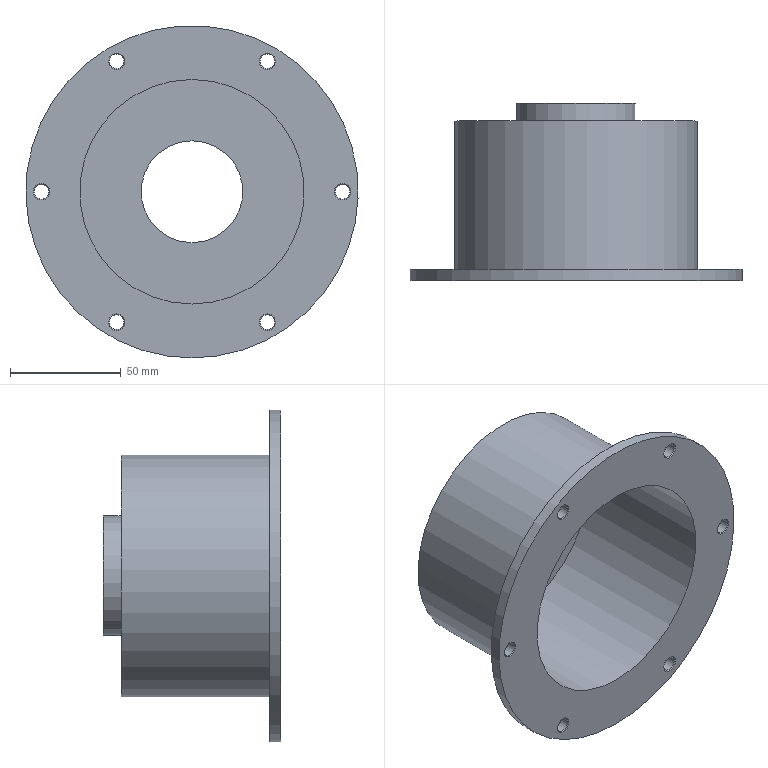Part | NX | features DATUM_CSYS 8, SKETCH 7, EXTRACT_DATUM_AXIS 6, EXTRACT_FACE 6, HOLE PACKAGE 6, SIMPLE HOLE 6, Instance Feature 5, Pattern Feature 1, SWP104 1 | 1 solid | 28 faces | box 150 x 80 x 150 mm | volume 166346 mm3 | cone 12 | cylinder 11 | plane 5 | commonest cylinder face diameters 6.6 x6 46 x1 54 x1 101.387 x1 109.387 x1 150 x1
STEP:
#1=CARTESIAN_POINT('',(0.,72.,-54.693));
#2=VERTEX_POINT('',#1);
#3=CARTESIAN_POINT('',(0.,72.,0.));
#4=DIRECTION('',(0.,-1.,0.));
#5=DIRECTION('',(0.,0.,-1.));
#6=AXIS2_PLACEMENT_3D('',#3,#4,#5);
#7=CIRCLE('',#6,54.693);
#8=EDGE_CURVE('',#2,#2,#7,.T.);
#9=ORIENTED_EDGE('',*,*,#8,.T.);
#10=EDGE_LOOP('',(#9));
#11=FACE_BOUND('',#10,.T.);
#12=CARTESIAN_POINT('',(0.,5.,-54.693));
#13=VERTEX_POINT('',#12);
#14=CARTESIAN_POINT('',(0.,5.,0.));
#15=DIRECTION('',(0.,-1.,0.));
#16=DIRECTION('',(0.,0.,-1.));
#17=AXIS2_PLACEMENT_3D('',#14,#15,#16);
#18=CIRCLE('',#17,54.693);
#19=EDGE_CURVE('',#13,#13,#18,.T.);
#20=ORIENTED_EDGE('',*,*,#19,.F.);
#21=EDGE_LOOP('',(#20));
#22=FACE_BOUND('',#21,.T.);
#23=CARTESIAN_POINT('',(0.,0.,0.));
#24=DIRECTION('',(0.,-1.,0.));
#25=DIRECTION('',(0.,0.,-1.));
#26=AXIS2_PLACEMENT_3D('',#23,#24,#25);
#27=CYLINDRICAL_SURFACE('',#26,54.693);
#28=ADVANCED_FACE('',(#11,#22),#27,.T.);
#29=CARTESIAN_POINT('',(0.,72.,-27.));
#30=VERTEX_POINT('',#29);
#31=CARTESIAN_POINT('',(0.,72.,0.));
#32=DIRECTION('',(0.,-1.,0.));
#33=DIRECTION('',(0.,0.,-1.));
#34=AXIS2_PLACEMENT_3D('',#31,#32,#33);
#35=CIRCLE('',#34,27.);
#36=EDGE_CURVE('',#30,#30,#35,.T.);
#37=ORIENTED_EDGE('',*,*,#36,.T.);
#38=EDGE_LOOP('',(#37));
#39=FACE_BOUND('',#38,.T.);
#40=ORIENTED_EDGE('',*,*,#8,.F.);
#41=EDGE_LOOP('',(#40));
#42=FACE_BOUND('',#41,.T.);
#43=CARTESIAN_POINT('',(54.693,72.,0.));
#44=DIRECTION('',(0.,1.,0.));
#45=DIRECTION('',(0.,0.,1.));
#46=AXIS2_PLACEMENT_3D('',#43,#44,#45);
#47=PLANE('',#46);
#48=ADVANCED_FACE('',(#39,#42),#47,.T.);
#49=CARTESIAN_POINT('',(0.,80.,-27.));
#50=VERTEX_POINT('',#49);
#51=CARTESIAN_POINT('',(0.,80.,0.));
#52=DIRECTION('',(0.,-1.,0.));
#53=DIRECTION('',(0.,0.,-1.));
#54=AXIS2_PLACEMENT_3D('',#51,#52,#53);
#55=CIRCLE('',#54,27.);
#56=EDGE_CURVE('',#50,#50,#55,.T.);
#57=ORIENTED_EDGE('',*,*,#56,.T.);
#58=EDGE_LOOP('',(#57));
#59=FACE_BOUND('',#58,.T.);
#60=ORIENTED_EDGE('',*,*,#36,.F.);
#61=EDGE_LOOP('',(#60));
#62=FACE_BOUND('',#61,.T.);
#63=CARTESIAN_POINT('',(0.,0.,0.));
#64=DIRECTION('',(0.,-1.,0.));
#65=DIRECTION('',(0.,0.,-1.));
#66=AXIS2_PLACEMENT_3D('',#63,#64,#65);
#67=CYLINDRICAL_SURFACE('',#66,27.);
#68=ADVANCED_FACE('',(#59,#62),#67,.T.);
#69=CARTESIAN_POINT('',(0.,80.,-23.));
#70=VERTEX_POINT('',#69);
#71=CARTESIAN_POINT('',(0.,80.,0.));
#72=DIRECTION('',(0.,-1.,0.));
#73=DIRECTION('',(0.,0.,-1.));
#74=AXIS2_PLACEMENT_3D('',#71,#72,#73);
#75=CIRCLE('',#74,23.);
#76=EDGE_CURVE('',#70,#70,#75,.T.);
#77=ORIENTED_EDGE('',*,*,#76,.T.);
#78=EDGE_LOOP('',(#77));
#79=FACE_BOUND('',#78,.T.);
#80=ORIENTED_EDGE('',*,*,#56,.F.);
#81=EDGE_LOOP('',(#80));
#82=FACE_BOUND('',#81,.T.);
#83=CARTESIAN_POINT('',(27.,80.,0.));
#84=DIRECTION('',(0.,1.,0.));
#85=DIRECTION('',(0.,0.,1.));
#86=AXIS2_PLACEMENT_3D('',#83,#84,#85);
#87=PLANE('',#86);
#88=ADVANCED_FACE('',(#79,#82),#87,.T.);
#89=CARTESIAN_POINT('',(0.,68.,-23.));
#90=VERTEX_POINT('',#89);
#91=CARTESIAN_POINT('',(0.,68.,0.));
#92=DIRECTION('',(0.,-1.,0.));
#93=DIRECTION('',(0.,0.,-1.));
#94=AXIS2_PLACEMENT_3D('',#91,#92,#93);
#95=CIRCLE('',#94,23.);
#96=EDGE_CURVE('',#90,#90,#95,.T.);
#97=ORIENTED_EDGE('',*,*,#96,.T.);
#98=EDGE_LOOP('',(#97));
#99=FACE_BOUND('',#98,.T.);
#100=ORIENTED_EDGE('',*,*,#76,.F.);
#101=EDGE_LOOP('',(#100));
#102=FACE_BOUND('',#101,.T.);
#103=CARTESIAN_POINT('',(0.,0.,0.));
#104=DIRECTION('',(0.,-1.,0.));
#105=DIRECTION('',(0.,0.,-1.));
#106=AXIS2_PLACEMENT_3D('',#103,#104,#105);
#107=CYLINDRICAL_SURFACE('',#106,23.);
#108=ADVANCED_FACE('',(#99,#102),#107,.F.);
#109=CARTESIAN_POINT('',(0.,68.,-50.693));
#110=VERTEX_POINT('',#109);
#111=CARTESIAN_POINT('',(0.,68.,0.));
#112=DIRECTION('',(0.,-1.,0.));
#113=DIRECTION('',(0.,0.,-1.));
#114=AXIS2_PLACEMENT_3D('',#111,#112,#113);
#115=CIRCLE('',#114,50.693);
#116=EDGE_CURVE('',#110,#110,#115,.T.);
#117=ORIENTED_EDGE('',*,*,#116,.T.);
#118=EDGE_LOOP('',(#117));
#119=FACE_BOUND('',#118,.T.);
#120=ORIENTED_EDGE('',*,*,#96,.F.);
#121=EDGE_LOOP('',(#120));
#122=FACE_BOUND('',#121,.T.);
#123=CARTESIAN_POINT('',(23.,68.,0.));
#124=DIRECTION('',(0.,-1.,0.));
#125=DIRECTION('',(0.,0.,-1.));
#126=AXIS2_PLACEMENT_3D('',#123,#124,#125);
#127=PLANE('',#126);
#128=ADVANCED_FACE('',(#119,#122),#127,.T.);
#129=CARTESIAN_POINT('',(0.,0.,-50.693));
#130=VERTEX_POINT('',#129);
#131=CARTESIAN_POINT('',(0.,0.,0.));
#132=DIRECTION('',(0.,-1.,0.));
#133=DIRECTION('',(0.,0.,-1.));
#134=AXIS2_PLACEMENT_3D('',#131,#132,#133);
#135=CIRCLE('',#134,50.693);
#136=EDGE_CURVE('',#130,#130,#135,.T.);
#137=ORIENTED_EDGE('',*,*,#136,.T.);
#138=EDGE_LOOP('',(#137));
#139=FACE_BOUND('',#138,.T.);
#140=ORIENTED_EDGE('',*,*,#116,.F.);
#141=EDGE_LOOP('',(#140));
#142=FACE_BOUND('',#141,.T.);
#143=CARTESIAN_POINT('',(0.,0.,0.));
#144=DIRECTION('',(0.,-1.,0.));
#145=DIRECTION('',(0.,0.,-1.));
#146=AXIS2_PLACEMENT_3D('',#143,#144,#145);
#147=CYLINDRICAL_SURFACE('',#146,50.693);
#148=ADVANCED_FACE('',(#139,#142),#147,.F.);
#149=CARTESIAN_POINT('',(34.,0.,55.19));
#150=VERTEX_POINT('',#149);
#151=CARTESIAN_POINT('',(34.,0.,58.89));
#152=DIRECTION('',(0.,-1.,0.));
#153=DIRECTION('',(0.,0.,-1.));
#154=AXIS2_PLACEMENT_3D('',#151,#152,#153);
#155=CIRCLE('',#154,3.7);
#156=EDGE_CURVE('',#150,#150,#155,.F.);
#157=ORIENTED_EDGE('',*,*,#156,.T.);
#158=EDGE_LOOP('',(#157));
#159=FACE_BOUND('',#158,.T.);
#160=CARTESIAN_POINT('',(-34.,0.,55.19));
#161=VERTEX_POINT('',#160);
#162=CARTESIAN_POINT('',(-34.,0.,58.89));
#163=DIRECTION('',(0.,-1.,0.));
#164=DIRECTION('',(0.,0.,-1.));
#165=AXIS2_PLACEMENT_3D('',#162,#163,#164);
#166=CIRCLE('',#165,3.7);
#167=EDGE_CURVE('',#161,#161,#166,.F.);
#168=ORIENTED_EDGE('',*,*,#167,.T.);
#169=EDGE_LOOP('',(#168));
#170=FACE_BOUND('',#169,.T.);
#171=CARTESIAN_POINT('',(-68.,0.,-3.7));
#172=VERTEX_POINT('',#171);
#173=CARTESIAN_POINT('',(-68.,0.,0.));
#174=DIRECTION('',(0.,-1.,0.));
#175=DIRECTION('',(0.,0.,-1.));
#176=AXIS2_PLACEMENT_3D('',#173,#174,#175);
#177=CIRCLE('',#176,3.7);
#178=EDGE_CURVE('',#172,#172,#177,.F.);
#179=ORIENTED_EDGE('',*,*,#178,.T.);
#180=EDGE_LOOP('',(#179));
#181=FACE_BOUND('',#180,.T.);
#182=CARTESIAN_POINT('',(-34.,0.,-62.59));
#183=VERTEX_POINT('',#182);
#184=CARTESIAN_POINT('',(-34.,0.,-58.89));
#185=DIRECTION('',(0.,-1.,0.));
#186=DIRECTION('',(0.,0.,-1.));
#187=AXIS2_PLACEMENT_3D('',#184,#185,#186);
#188=CIRCLE('',#187,3.7);
#189=EDGE_CURVE('',#183,#183,#188,.F.);
#190=ORIENTED_EDGE('',*,*,#189,.T.);
#191=EDGE_LOOP('',(#190));
#192=FACE_BOUND('',#191,.T.);
#193=CARTESIAN_POINT('',(34.,0.,-62.59));
#194=VERTEX_POINT('',#193);
#195=CARTESIAN_POINT('',(34.,0.,-58.89));
#196=DIRECTION('',(0.,-1.,0.));
#197=DIRECTION('',(0.,0.,-1.));
#198=AXIS2_PLACEMENT_3D('',#195,#196,#197);
#199=CIRCLE('',#198,3.7);
#200=EDGE_CURVE('',#194,#194,#199,.F.);
#201=ORIENTED_EDGE('',*,*,#200,.T.);
#202=EDGE_LOOP('',(#201));
#203=FACE_BOUND('',#202,.T.);
#204=CARTESIAN_POINT('',(68.,0.,-3.7));
#205=VERTEX_POINT('',#204);
#206=CARTESIAN_POINT('',(68.,0.,0.));
#207=DIRECTION('',(0.,-1.,0.));
#208=DIRECTION('',(0.,0.,-1.));
#209=AXIS2_PLACEMENT_3D('',#206,#207,#208);
#210=CIRCLE('',#209,3.7);
#211=EDGE_CURVE('',#205,#205,#210,.F.);
#212=ORIENTED_EDGE('',*,*,#211,.T.);
#213=EDGE_LOOP('',(#212));
#214=FACE_BOUND('',#213,.T.);
#215=CARTESIAN_POINT('',(0.,0.,-75.));
#216=VERTEX_POINT('',#215);
#217=CARTESIAN_POINT('',(0.,0.,0.));
#218=DIRECTION('',(0.,-1.,0.));
#219=DIRECTION('',(0.,0.,-1.));
#220=AXIS2_PLACEMENT_3D('',#217,#218,#219);
#221=CIRCLE('',#220,75.);
#222=EDGE_CURVE('',#216,#216,#221,.T.);
#223=ORIENTED_EDGE('',*,*,#222,.T.);
#224=EDGE_LOOP('',(#223));
#225=FACE_BOUND('',#224,.T.);
#226=ORIENTED_EDGE('',*,*,#136,.F.);
#227=EDGE_LOOP('',(#226));
#228=FACE_BOUND('',#227,.T.);
#229=CARTESIAN_POINT('',(50.693,0.,0.));
#230=DIRECTION('',(0.,-1.,0.));
#231=DIRECTION('',(0.,0.,-1.));
#232=AXIS2_PLACEMENT_3D('',#229,#230,#231);
#233=PLANE('',#232);
#234=ADVANCED_FACE('',(#159,#170,#181,#192,#203,#214,#225,#228),#233,.T.);
#235=CARTESIAN_POINT('',(0.,5.,-75.));
#236=VERTEX_POINT('',#235);
#237=CARTESIAN_POINT('',(0.,5.,0.));
#238=DIRECTION('',(0.,-1.,0.));
#239=DIRECTION('',(0.,0.,-1.));
#240=AXIS2_PLACEMENT_3D('',#237,#238,#239);
#241=CIRCLE('',#240,75.);
#242=EDGE_CURVE('',#236,#236,#241,.T.);
#243=ORIENTED_EDGE('',*,*,#242,.T.);
#244=EDGE_LOOP('',(#243));
#245=FACE_BOUND('',#244,.T.);
#246=ORIENTED_EDGE('',*,*,#222,.F.);
#247=EDGE_LOOP('',(#246));
#248=FACE_BOUND('',#247,.T.);
#249=CARTESIAN_POINT('',(0.,0.,0.));
#250=DIRECTION('',(0.,-1.,0.));
#251=DIRECTION('',(0.,0.,-1.));
#252=AXIS2_PLACEMENT_3D('',#249,#250,#251);
#253=CYLINDRICAL_SURFACE('',#252,75.);
#254=ADVANCED_FACE('',(#245,#248),#253,.T.);
#255=CARTESIAN_POINT('',(34.,5.,62.59));
#256=VERTEX_POINT('',#255);
#257=CARTESIAN_POINT('',(34.,5.,58.89));
#258=DIRECTION('',(0.,1.,0.));
#259=DIRECTION('',(0.,0.,1.));
#260=AXIS2_PLACEMENT_3D('',#257,#258,#259);
#261=CIRCLE('',#260,3.7);
#262=EDGE_CURVE('',#256,#256,#261,.F.);
#263=ORIENTED_EDGE('',*,*,#262,.T.);
#264=EDGE_LOOP('',(#263));
#265=FACE_BOUND('',#264,.T.);
#266=CARTESIAN_POINT('',(-34.,5.,62.59));
#267=VERTEX_POINT('',#266);
#268=CARTESIAN_POINT('',(-34.,5.,58.89));
#269=DIRECTION('',(0.,1.,0.));
#270=DIRECTION('',(0.,0.,1.));
#271=AXIS2_PLACEMENT_3D('',#268,#269,#270);
#272=CIRCLE('',#271,3.7);
#273=EDGE_CURVE('',#267,#267,#272,.F.);
#274=ORIENTED_EDGE('',*,*,#273,.T.);
#275=EDGE_LOOP('',(#274));
#276=FACE_BOUND('',#275,.T.);
#277=CARTESIAN_POINT('',(-68.,5.,3.7));
#278=VERTEX_POINT('',#277);
#279=CARTESIAN_POINT('',(-68.,5.,0.));
#280=DIRECTION('',(0.,1.,0.));
#281=DIRECTION('',(0.,0.,1.));
#282=AXIS2_PLACEMENT_3D('',#279,#280,#281);
#283=CIRCLE('',#282,3.7);
#284=EDGE_CURVE('',#278,#278,#283,.F.);
#285=ORIENTED_EDGE('',*,*,#284,.T.);
#286=EDGE_LOOP('',(#285));
#287=FACE_BOUND('',#286,.T.);
#288=CARTESIAN_POINT('',(-34.,5.,-55.19));
#289=VERTEX_POINT('',#288);
#290=CARTESIAN_POINT('',(-34.,5.,-58.89));
#291=DIRECTION('',(0.,1.,0.));
#292=DIRECTION('',(0.,0.,1.));
#293=AXIS2_PLACEMENT_3D('',#290,#291,#292);
#294=CIRCLE('',#293,3.7);
#295=EDGE_CURVE('',#289,#289,#294,.F.);
#296=ORIENTED_EDGE('',*,*,#295,.T.);
#297=EDGE_LOOP('',(#296));
#298=FACE_BOUND('',#297,.T.);
#299=CARTESIAN_POINT('',(34.,5.,-55.19));
#300=VERTEX_POINT('',#299);
#301=CARTESIAN_POINT('',(34.,5.,-58.89));
#302=DIRECTION('',(0.,1.,0.));
#303=DIRECTION('',(0.,0.,1.));
#304=AXIS2_PLACEMENT_3D('',#301,#302,#303);
#305=CIRCLE('',#304,3.7);
#306=EDGE_CURVE('',#300,#300,#305,.F.);
#307=ORIENTED_EDGE('',*,*,#306,.T.);
#308=EDGE_LOOP('',(#307));
#309=FACE_BOUND('',#308,.T.);
#310=CARTESIAN_POINT('',(68.,5.,3.7));
#311=VERTEX_POINT('',#310);
#312=CARTESIAN_POINT('',(68.,5.,0.));
#313=DIRECTION('',(0.,1.,0.));
#314=DIRECTION('',(0.,0.,1.));
#315=AXIS2_PLACEMENT_3D('',#312,#313,#314);
#316=CIRCLE('',#315,3.7);
#317=EDGE_CURVE('',#311,#311,#316,.F.);
#318=ORIENTED_EDGE('',*,*,#317,.T.);
#319=EDGE_LOOP('',(#318));
#320=FACE_BOUND('',#319,.T.);
#321=ORIENTED_EDGE('',*,*,#19,.T.);
#322=EDGE_LOOP('',(#321));
#323=FACE_BOUND('',#322,.T.);
#324=ORIENTED_EDGE('',*,*,#242,.F.);
#325=EDGE_LOOP('',(#324));
#326=FACE_BOUND('',#325,.T.);
#327=CARTESIAN_POINT('',(75.,5.,0.));
#328=DIRECTION('',(0.,1.,0.));
#329=DIRECTION('',(0.,0.,1.));
#330=AXIS2_PLACEMENT_3D('',#327,#328,#329);
#331=PLANE('',#330);
#332=ADVANCED_FACE('',(#265,#276,#287,#298,#309,#320,#323,#326),#331,.T.);
#333=CARTESIAN_POINT('',(68.,0.4,-3.3));
#334=VERTEX_POINT('',#333);
#335=CARTESIAN_POINT('',(68.,0.4,0.));
#336=DIRECTION('',(0.,-1.,0.));
#337=DIRECTION('',(0.,0.,-1.));
#338=AXIS2_PLACEMENT_3D('',#335,#336,#337);
#339=CIRCLE('',#338,3.3);
#340=EDGE_CURVE('',#334,#334,#339,.T.);
#341=ORIENTED_EDGE('',*,*,#340,.T.);
#342=EDGE_LOOP('',(#341));
#343=FACE_BOUND('',#342,.T.);
#344=CARTESIAN_POINT('',(68.,4.6,3.3));
#345=VERTEX_POINT('',#344);
#346=CARTESIAN_POINT('',(68.,4.6,0.));
#347=DIRECTION('',(0.,1.,0.));
#348=DIRECTION('',(0.,0.,1.));
#349=AXIS2_PLACEMENT_3D('',#346,#347,#348);
#350=CIRCLE('',#349,3.3);
#351=EDGE_CURVE('',#345,#345,#350,.T.);
#352=ORIENTED_EDGE('',*,*,#351,.T.);
#353=EDGE_LOOP('',(#352));
#354=FACE_BOUND('',#353,.T.);
#355=CARTESIAN_POINT('',(68.,5.,0.));
#356=DIRECTION('',(0.,-1.,0.));
#357=DIRECTION('',(0.,0.,-1.));
#358=AXIS2_PLACEMENT_3D('',#355,#356,#357);
#359=CYLINDRICAL_SURFACE('',#358,3.3);
#360=ADVANCED_FACE('',(#343,#354),#359,.F.);
#361=ORIENTED_EDGE('',*,*,#351,.F.);
#362=EDGE_LOOP('',(#361));
#363=FACE_BOUND('',#362,.T.);
#364=ORIENTED_EDGE('',*,*,#317,.F.);
#365=EDGE_LOOP('',(#364));
#366=FACE_BOUND('',#365,.T.);
#367=CARTESIAN_POINT('',(68.,5.,0.));
#368=DIRECTION('',(0.,1.,0.));
#369=DIRECTION('',(0.,0.,1.));
#370=AXIS2_PLACEMENT_3D('',#367,#368,#369);
#371=CONICAL_SURFACE('',#370,3.7,0.7854);
#372=ADVANCED_FACE('',(#363,#366),#371,.F.);
#373=ORIENTED_EDGE('',*,*,#211,.F.);
#374=EDGE_LOOP('',(#373));
#375=FACE_BOUND('',#374,.T.);
#376=ORIENTED_EDGE('',*,*,#340,.F.);
#377=EDGE_LOOP('',(#376));
#378=FACE_BOUND('',#377,.T.);
#379=CARTESIAN_POINT('',(68.,0.4,0.));
#380=DIRECTION('',(0.,-1.,0.));
#381=DIRECTION('',(0.,0.,-1.));
#382=AXIS2_PLACEMENT_3D('',#379,#380,#381);
#383=CONICAL_SURFACE('',#382,3.3,0.7854);
#384=ADVANCED_FACE('',(#375,#378),#383,.F.);
#385=CARTESIAN_POINT('',(34.,0.4,-62.19));
#386=VERTEX_POINT('',#385);
#387=CARTESIAN_POINT('',(34.,0.4,-58.89));
#388=DIRECTION('',(0.,-1.,0.));
#389=DIRECTION('',(0.,0.,-1.));
#390=AXIS2_PLACEMENT_3D('',#387,#388,#389);
#391=CIRCLE('',#390,3.3);
#392=EDGE_CURVE('',#386,#386,#391,.T.);
#393=ORIENTED_EDGE('',*,*,#392,.T.);
#394=EDGE_LOOP('',(#393));
#395=FACE_BOUND('',#394,.T.);
#396=CARTESIAN_POINT('',(34.,4.6,-55.59));
#397=VERTEX_POINT('',#396);
#398=CARTESIAN_POINT('',(34.,4.6,-58.89));
#399=DIRECTION('',(0.,1.,0.));
#400=DIRECTION('',(0.,0.,1.));
#401=AXIS2_PLACEMENT_3D('',#398,#399,#400);
#402=CIRCLE('',#401,3.3);
#403=EDGE_CURVE('',#397,#397,#402,.T.);
#404=ORIENTED_EDGE('',*,*,#403,.T.);
#405=EDGE_LOOP('',(#404));
#406=FACE_BOUND('',#405,.T.);
#407=CARTESIAN_POINT('',(34.,5.,-58.89));
#408=DIRECTION('',(0.,-1.,0.));
#409=DIRECTION('',(0.,0.,-1.));
#410=AXIS2_PLACEMENT_3D('',#407,#408,#409);
#411=CYLINDRICAL_SURFACE('',#410,3.3);
#412=ADVANCED_FACE('',(#395,#406),#411,.F.);
#413=ORIENTED_EDGE('',*,*,#403,.F.);
#414=EDGE_LOOP('',(#413));
#415=FACE_BOUND('',#414,.T.);
#416=ORIENTED_EDGE('',*,*,#306,.F.);
#417=EDGE_LOOP('',(#416));
#418=FACE_BOUND('',#417,.T.);
#419=CARTESIAN_POINT('',(34.,5.,-58.89));
#420=DIRECTION('',(0.,1.,0.));
#421=DIRECTION('',(0.,0.,1.));
#422=AXIS2_PLACEMENT_3D('',#419,#420,#421);
#423=CONICAL_SURFACE('',#422,3.7,0.7854);
#424=ADVANCED_FACE('',(#415,#418),#423,.F.);
#425=ORIENTED_EDGE('',*,*,#200,.F.);
#426=EDGE_LOOP('',(#425));
#427=FACE_BOUND('',#426,.T.);
#428=ORIENTED_EDGE('',*,*,#392,.F.);
#429=EDGE_LOOP('',(#428));
#430=FACE_BOUND('',#429,.T.);
#431=CARTESIAN_POINT('',(34.,0.4,-58.89));
#432=DIRECTION('',(0.,-1.,0.));
#433=DIRECTION('',(0.,0.,-1.));
#434=AXIS2_PLACEMENT_3D('',#431,#432,#433);
#435=CONICAL_SURFACE('',#434,3.3,0.7854);
#436=ADVANCED_FACE('',(#427,#430),#435,.F.);
#437=CARTESIAN_POINT('',(-34.,0.4,-62.19));
#438=VERTEX_POINT('',#437);
#439=CARTESIAN_POINT('',(-34.,0.4,-58.89));
#440=DIRECTION('',(0.,-1.,0.));
#441=DIRECTION('',(0.,0.,-1.));
#442=AXIS2_PLACEMENT_3D('',#439,#440,#441);
#443=CIRCLE('',#442,3.3);
#444=EDGE_CURVE('',#438,#438,#443,.T.);
#445=ORIENTED_EDGE('',*,*,#444,.T.);
#446=EDGE_LOOP('',(#445));
#447=FACE_BOUND('',#446,.T.);
#448=CARTESIAN_POINT('',(-34.,4.6,-55.59));
#449=VERTEX_POINT('',#448);
#450=CARTESIAN_POINT('',(-34.,4.6,-58.89));
#451=DIRECTION('',(0.,1.,0.));
#452=DIRECTION('',(0.,0.,1.));
#453=AXIS2_PLACEMENT_3D('',#450,#451,#452);
#454=CIRCLE('',#453,3.3);
#455=EDGE_CURVE('',#449,#449,#454,.T.);
#456=ORIENTED_EDGE('',*,*,#455,.T.);
#457=EDGE_LOOP('',(#456));
#458=FACE_BOUND('',#457,.T.);
#459=CARTESIAN_POINT('',(-34.,5.,-58.89));
#460=DIRECTION('',(0.,-1.,0.));
#461=DIRECTION('',(0.,0.,-1.));
#462=AXIS2_PLACEMENT_3D('',#459,#460,#461);
#463=CYLINDRICAL_SURFACE('',#462,3.3);
#464=ADVANCED_FACE('',(#447,#458),#463,.F.);
#465=ORIENTED_EDGE('',*,*,#455,.F.);
#466=EDGE_LOOP('',(#465));
#467=FACE_BOUND('',#466,.T.);
#468=ORIENTED_EDGE('',*,*,#295,.F.);
#469=EDGE_LOOP('',(#468));
#470=FACE_BOUND('',#469,.T.);
#471=CARTESIAN_POINT('',(-34.,5.,-58.89));
#472=DIRECTION('',(0.,1.,0.));
#473=DIRECTION('',(0.,0.,1.));
#474=AXIS2_PLACEMENT_3D('',#471,#472,#473);
#475=CONICAL_SURFACE('',#474,3.7,0.7854);
#476=ADVANCED_FACE('',(#467,#470),#475,.F.);
#477=ORIENTED_EDGE('',*,*,#189,.F.);
#478=EDGE_LOOP('',(#477));
#479=FACE_BOUND('',#478,.T.);
#480=ORIENTED_EDGE('',*,*,#444,.F.);
#481=EDGE_LOOP('',(#480));
#482=FACE_BOUND('',#481,.T.);
#483=CARTESIAN_POINT('',(-34.,0.4,-58.89));
#484=DIRECTION('',(0.,-1.,0.));
#485=DIRECTION('',(0.,0.,-1.));
#486=AXIS2_PLACEMENT_3D('',#483,#484,#485);
#487=CONICAL_SURFACE('',#486,3.3,0.7854);
#488=ADVANCED_FACE('',(#479,#482),#487,.F.);
#489=CARTESIAN_POINT('',(-68.,0.4,-3.3));
#490=VERTEX_POINT('',#489);
#491=CARTESIAN_POINT('',(-68.,0.4,0.));
#492=DIRECTION('',(0.,-1.,0.));
#493=DIRECTION('',(0.,0.,-1.));
#494=AXIS2_PLACEMENT_3D('',#491,#492,#493);
#495=CIRCLE('',#494,3.3);
#496=EDGE_CURVE('',#490,#490,#495,.T.);
#497=ORIENTED_EDGE('',*,*,#496,.T.);
#498=EDGE_LOOP('',(#497));
#499=FACE_BOUND('',#498,.T.);
#500=CARTESIAN_POINT('',(-68.,4.6,3.3));
#501=VERTEX_POINT('',#500);
#502=CARTESIAN_POINT('',(-68.,4.6,0.));
#503=DIRECTION('',(0.,1.,0.));
#504=DIRECTION('',(0.,0.,1.));
#505=AXIS2_PLACEMENT_3D('',#502,#503,#504);
#506=CIRCLE('',#505,3.3);
#507=EDGE_CURVE('',#501,#501,#506,.T.);
#508=ORIENTED_EDGE('',*,*,#507,.T.);
#509=EDGE_LOOP('',(#508));
#510=FACE_BOUND('',#509,.T.);
#511=CARTESIAN_POINT('',(-68.,5.,0.));
#512=DIRECTION('',(0.,-1.,0.));
#513=DIRECTION('',(0.,0.,-1.));
#514=AXIS2_PLACEMENT_3D('',#511,#512,#513);
#515=CYLINDRICAL_SURFACE('',#514,3.3);
#516=ADVANCED_FACE('',(#499,#510),#515,.F.);
#517=ORIENTED_EDGE('',*,*,#507,.F.);
#518=EDGE_LOOP('',(#517));
#519=FACE_BOUND('',#518,.T.);
#520=ORIENTED_EDGE('',*,*,#284,.F.);
#521=EDGE_LOOP('',(#520));
#522=FACE_BOUND('',#521,.T.);
#523=CARTESIAN_POINT('',(-68.,5.,0.));
#524=DIRECTION('',(0.,1.,0.));
#525=DIRECTION('',(0.,0.,1.));
#526=AXIS2_PLACEMENT_3D('',#523,#524,#525);
#527=CONICAL_SURFACE('',#526,3.7,0.7854);
#528=ADVANCED_FACE('',(#519,#522),#527,.F.);
#529=ORIENTED_EDGE('',*,*,#178,.F.);
#530=EDGE_LOOP('',(#529));
#531=FACE_BOUND('',#530,.T.);
#532=ORIENTED_EDGE('',*,*,#496,.F.);
#533=EDGE_LOOP('',(#532));
#534=FACE_BOUND('',#533,.T.);
#535=CARTESIAN_POINT('',(-68.,0.4,0.));
#536=DIRECTION('',(0.,-1.,0.));
#537=DIRECTION('',(0.,0.,-1.));
#538=AXIS2_PLACEMENT_3D('',#535,#536,#537);
#539=CONICAL_SURFACE('',#538,3.3,0.7854);
#540=ADVANCED_FACE('',(#531,#534),#539,.F.);
#541=CARTESIAN_POINT('',(-34.,0.4,55.59));
#542=VERTEX_POINT('',#541);
#543=CARTESIAN_POINT('',(-34.,0.4,58.89));
#544=DIRECTION('',(0.,-1.,0.));
#545=DIRECTION('',(0.,0.,-1.));
#546=AXIS2_PLACEMENT_3D('',#543,#544,#545);
#547=CIRCLE('',#546,3.3);
#548=EDGE_CURVE('',#542,#542,#547,.T.);
#549=ORIENTED_EDGE('',*,*,#548,.T.);
#550=EDGE_LOOP('',(#549));
#551=FACE_BOUND('',#550,.T.);
#552=CARTESIAN_POINT('',(-34.,4.6,62.19));
#553=VERTEX_POINT('',#552);
#554=CARTESIAN_POINT('',(-34.,4.6,58.89));
#555=DIRECTION('',(0.,1.,0.));
#556=DIRECTION('',(0.,0.,1.));
#557=AXIS2_PLACEMENT_3D('',#554,#555,#556);
#558=CIRCLE('',#557,3.3);
#559=EDGE_CURVE('',#553,#553,#558,.T.);
#560=ORIENTED_EDGE('',*,*,#559,.T.);
#561=EDGE_LOOP('',(#560));
#562=FACE_BOUND('',#561,.T.);
#563=CARTESIAN_POINT('',(-34.,5.,58.89));
#564=DIRECTION('',(0.,-1.,0.));
#565=DIRECTION('',(0.,0.,-1.));
#566=AXIS2_PLACEMENT_3D('',#563,#564,#565);
#567=CYLINDRICAL_SURFACE('',#566,3.3);
#568=ADVANCED_FACE('',(#551,#562),#567,.F.);
#569=ORIENTED_EDGE('',*,*,#559,.F.);
#570=EDGE_LOOP('',(#569));
#571=FACE_BOUND('',#570,.T.);
#572=ORIENTED_EDGE('',*,*,#273,.F.);
#573=EDGE_LOOP('',(#572));
#574=FACE_BOUND('',#573,.T.);
#575=CARTESIAN_POINT('',(-34.,5.,58.89));
#576=DIRECTION('',(0.,1.,0.));
#577=DIRECTION('',(0.,0.,1.));
#578=AXIS2_PLACEMENT_3D('',#575,#576,#577);
#579=CONICAL_SURFACE('',#578,3.7,0.7854);
#580=ADVANCED_FACE('',(#571,#574),#579,.F.);
#581=ORIENTED_EDGE('',*,*,#167,.F.);
#582=EDGE_LOOP('',(#581));
#583=FACE_BOUND('',#582,.T.);
#584=ORIENTED_EDGE('',*,*,#548,.F.);
#585=EDGE_LOOP('',(#584));
#586=FACE_BOUND('',#585,.T.);
#587=CARTESIAN_POINT('',(-34.,0.4,58.89));
#588=DIRECTION('',(0.,-1.,0.));
#589=DIRECTION('',(0.,0.,-1.));
#590=AXIS2_PLACEMENT_3D('',#587,#588,#589);
#591=CONICAL_SURFACE('',#590,3.3,0.7854);
#592=ADVANCED_FACE('',(#583,#586),#591,.F.);
#593=CARTESIAN_POINT('',(34.,0.4,55.59));
#594=VERTEX_POINT('',#593);
#595=CARTESIAN_POINT('',(34.,0.4,58.89));
#596=DIRECTION('',(0.,-1.,0.));
#597=DIRECTION('',(0.,0.,-1.));
#598=AXIS2_PLACEMENT_3D('',#595,#596,#597);
#599=CIRCLE('',#598,3.3);
#600=EDGE_CURVE('',#594,#594,#599,.T.);
#601=ORIENTED_EDGE('',*,*,#600,.T.);
#602=EDGE_LOOP('',(#601));
#603=FACE_BOUND('',#602,.T.);
#604=CARTESIAN_POINT('',(34.,4.6,62.19));
#605=VERTEX_POINT('',#604);
#606=CARTESIAN_POINT('',(34.,4.6,58.89));
#607=DIRECTION('',(0.,1.,0.));
#608=DIRECTION('',(0.,0.,1.));
#609=AXIS2_PLACEMENT_3D('',#606,#607,#608);
#610=CIRCLE('',#609,3.3);
#611=EDGE_CURVE('',#605,#605,#610,.T.);
#612=ORIENTED_EDGE('',*,*,#611,.T.);
#613=EDGE_LOOP('',(#612));
#614=FACE_BOUND('',#613,.T.);
#615=CARTESIAN_POINT('',(34.,5.,58.89));
#616=DIRECTION('',(0.,-1.,0.));
#617=DIRECTION('',(0.,0.,-1.));
#618=AXIS2_PLACEMENT_3D('',#615,#616,#617);
#619=CYLINDRICAL_SURFACE('',#618,3.3);
#620=ADVANCED_FACE('',(#603,#614),#619,.F.);
#621=ORIENTED_EDGE('',*,*,#611,.F.);
#622=EDGE_LOOP('',(#621));
#623=FACE_BOUND('',#622,.T.);
#624=ORIENTED_EDGE('',*,*,#262,.F.);
#625=EDGE_LOOP('',(#624));
#626=FACE_BOUND('',#625,.T.);
#627=CARTESIAN_POINT('',(34.,5.,58.89));
#628=DIRECTION('',(0.,1.,0.));
#629=DIRECTION('',(0.,0.,1.));
#630=AXIS2_PLACEMENT_3D('',#627,#628,#629);
#631=CONICAL_SURFACE('',#630,3.7,0.7854);
#632=ADVANCED_FACE('',(#623,#626),#631,.F.);
#633=ORIENTED_EDGE('',*,*,#156,.F.);
#634=EDGE_LOOP('',(#633));
#635=FACE_BOUND('',#634,.T.);
#636=ORIENTED_EDGE('',*,*,#600,.F.);
#637=EDGE_LOOP('',(#636));
#638=FACE_BOUND('',#637,.T.);
#639=CARTESIAN_POINT('',(34.,0.4,58.89));
#640=DIRECTION('',(0.,-1.,0.));
#641=DIRECTION('',(0.,0.,-1.));
#642=AXIS2_PLACEMENT_3D('',#639,#640,#641);
#643=CONICAL_SURFACE('',#642,3.3,0.7854);
#644=ADVANCED_FACE('',(#635,#638),#643,.F.);
#645=CLOSED_SHELL('',(#28,#48,#68,#88,#108,#128,#148,#234,#254,#332,#360,#372,#384,#412,#424,#436,#464,#476,#488,#516,#528,#540,#568,#580,#592,#620,#632,#644));
#646=MANIFOLD_SOLID_BREP('',#645);
#647=(LENGTH_UNIT()NAMED_UNIT(*)SI_UNIT(.MILLI.,.METRE.));
#648=UNCERTAINTY_MEASURE_WITH_UNIT(LENGTH_MEASURE(0.00001),#647,'','');
#649=(NAMED_UNIT(*)PLANE_ANGLE_UNIT()SI_UNIT($,.RADIAN.));
#650=(NAMED_UNIT(*)SI_UNIT($,.STERADIAN.)SOLID_ANGLE_UNIT());
#651=(GEOMETRIC_REPRESENTATION_CONTEXT(3)GLOBAL_UNCERTAINTY_ASSIGNED_CONTEXT((#648))GLOBAL_UNIT_ASSIGNED_CONTEXT((#647,#649,#650))REPRESENTATION_CONTEXT('',''));
#652=ADVANCED_BREP_SHAPE_REPRESENTATION('',(#646),#651);